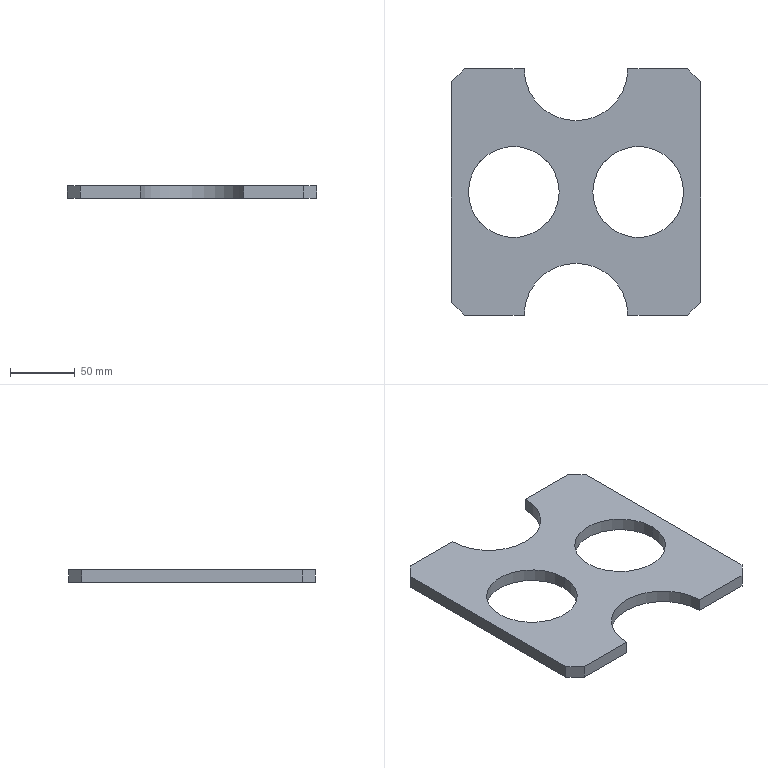Part | SolidWorks | features Extrusion 1 | 1 solid | 18 faces | box 192 x 190 x 10 mm | volume 235565 mm3 | plane 12 | cylinder 6 | commonest cylinder face diameters 70 x4 80 x2
STEP:
#1=CARTESIAN_POINT('',(109.,95.,10.));
#2=VERTEX_POINT('',#1);
#3=CARTESIAN_POINT('',(179.,95.,10.));
#4=VERTEX_POINT('',#3);
#5=CARTESIAN_POINT('',(144.,95.,10.));
#6=DIRECTION('',(0.,0.,1.));
#7=DIRECTION('',(1.,0.,0.));
#8=AXIS2_PLACEMENT_3D('',#5,#6,#7);
#9=CIRCLE('',#8,35.);
#10=EDGE_CURVE('',#2,#4,#9,.T.);
#11=ORIENTED_EDGE('',*,*,#10,.T.);
#12=CARTESIAN_POINT('',(179.,95.,0.));
#13=VERTEX_POINT('',#12);
#14=CARTESIAN_POINT('',(179.,95.,10.));
#15=DIRECTION('',(0.,0.,-1.));
#16=VECTOR('',#15,1000.);
#17=LINE('',#14,#16);
#18=EDGE_CURVE('',#4,#13,#17,.T.);
#19=ORIENTED_EDGE('',*,*,#18,.T.);
#20=CARTESIAN_POINT('',(109.,95.,0.));
#21=VERTEX_POINT('',#20);
#22=CARTESIAN_POINT('',(144.,95.,0.));
#23=DIRECTION('',(0.,0.,1.));
#24=DIRECTION('',(1.,0.,0.));
#25=AXIS2_PLACEMENT_3D('',#22,#23,#24);
#26=CIRCLE('',#25,35.);
#27=EDGE_CURVE('',#21,#13,#26,.T.);
#28=ORIENTED_EDGE('',*,*,#27,.F.);
#29=CARTESIAN_POINT('',(109.,95.,10.));
#30=DIRECTION('',(0.,0.,-1.));
#31=VECTOR('',#30,1000.);
#32=LINE('',#29,#31);
#33=EDGE_CURVE('',#2,#21,#32,.T.);
#34=ORIENTED_EDGE('',*,*,#33,.F.);
#35=EDGE_LOOP('',(#11,#19,#28,#34));
#36=FACE_OUTER_BOUND('',#35,.T.);
#37=CARTESIAN_POINT('',(144.,95.,10.));
#38=DIRECTION('',(0.,0.,-1.));
#39=DIRECTION('',(-1.,0.,0.));
#40=AXIS2_PLACEMENT_3D('',#37,#38,#39);
#41=CYLINDRICAL_SURFACE('',#40,35.);
#42=ADVANCED_FACE('',(#36),#41,.F.);
#43=CARTESIAN_POINT('',(13.,95.,10.));
#44=VERTEX_POINT('',#43);
#45=CARTESIAN_POINT('',(83.,95.,10.));
#46=VERTEX_POINT('',#45);
#47=CARTESIAN_POINT('',(48.,95.,10.));
#48=DIRECTION('',(0.,0.,1.));
#49=DIRECTION('',(1.,0.,0.));
#50=AXIS2_PLACEMENT_3D('',#47,#48,#49);
#51=CIRCLE('',#50,35.);
#52=EDGE_CURVE('',#44,#46,#51,.T.);
#53=ORIENTED_EDGE('',*,*,#52,.T.);
#54=CARTESIAN_POINT('',(83.,95.,0.));
#55=VERTEX_POINT('',#54);
#56=CARTESIAN_POINT('',(83.,95.,10.));
#57=DIRECTION('',(0.,0.,-1.));
#58=VECTOR('',#57,1000.);
#59=LINE('',#56,#58);
#60=EDGE_CURVE('',#46,#55,#59,.T.);
#61=ORIENTED_EDGE('',*,*,#60,.T.);
#62=CARTESIAN_POINT('',(13.,95.,0.));
#63=VERTEX_POINT('',#62);
#64=CARTESIAN_POINT('',(48.,95.,0.));
#65=DIRECTION('',(0.,0.,1.));
#66=DIRECTION('',(1.,0.,0.));
#67=AXIS2_PLACEMENT_3D('',#64,#65,#66);
#68=CIRCLE('',#67,35.);
#69=EDGE_CURVE('',#63,#55,#68,.T.);
#70=ORIENTED_EDGE('',*,*,#69,.F.);
#71=CARTESIAN_POINT('',(13.,95.,10.));
#72=DIRECTION('',(0.,0.,-1.));
#73=VECTOR('',#72,1000.);
#74=LINE('',#71,#73);
#75=EDGE_CURVE('',#44,#63,#74,.T.);
#76=ORIENTED_EDGE('',*,*,#75,.F.);
#77=EDGE_LOOP('',(#53,#61,#70,#76));
#78=FACE_OUTER_BOUND('',#77,.T.);
#79=CARTESIAN_POINT('',(48.,95.,10.));
#80=DIRECTION('',(0.,0.,-1.));
#81=DIRECTION('',(-1.,0.,0.));
#82=AXIS2_PLACEMENT_3D('',#79,#80,#81);
#83=CYLINDRICAL_SURFACE('',#82,35.);
#84=ADVANCED_FACE('',(#78),#83,.F.);
#85=ORIENTED_EDGE('',*,*,#52,.F.);
#86=CARTESIAN_POINT('',(48.,95.,10.));
#87=DIRECTION('',(0.,0.,1.));
#88=DIRECTION('',(1.,0.,0.));
#89=AXIS2_PLACEMENT_3D('',#86,#87,#88);
#90=CIRCLE('',#89,35.);
#91=EDGE_CURVE('',#46,#44,#90,.T.);
#92=ORIENTED_EDGE('',*,*,#91,.F.);
#93=EDGE_LOOP('',(#85,#92));
#94=FACE_BOUND('',#93,.T.);
#95=CARTESIAN_POINT('',(56.,0.,10.));
#96=VERTEX_POINT('',#95);
#97=CARTESIAN_POINT('',(136.,0.,10.));
#98=VERTEX_POINT('',#97);
#99=CARTESIAN_POINT('',(96.,0.,10.));
#100=DIRECTION('',(0.,0.,-1.));
#101=DIRECTION('',(1.,0.,0.));
#102=AXIS2_PLACEMENT_3D('',#99,#100,#101);
#103=CIRCLE('',#102,40.);
#104=EDGE_CURVE('',#96,#98,#103,.T.);
#105=ORIENTED_EDGE('',*,*,#104,.T.);
#106=CARTESIAN_POINT('',(182.,0.,10.));
#107=VERTEX_POINT('',#106);
#108=CARTESIAN_POINT('',(136.,0.,10.));
#109=DIRECTION('',(1.,0.,0.));
#110=VECTOR('',#109,1000.);
#111=LINE('',#108,#110);
#112=EDGE_CURVE('',#98,#107,#111,.T.);
#113=ORIENTED_EDGE('',*,*,#112,.T.);
#114=CARTESIAN_POINT('',(192.,10.,10.));
#115=VERTEX_POINT('',#114);
#116=CARTESIAN_POINT('',(182.,0.,10.));
#117=DIRECTION('',(0.7071,0.7071,0.));
#118=VECTOR('',#117,1000.);
#119=LINE('',#116,#118);
#120=EDGE_CURVE('',#107,#115,#119,.T.);
#121=ORIENTED_EDGE('',*,*,#120,.T.);
#122=CARTESIAN_POINT('',(192.,180.,10.));
#123=VERTEX_POINT('',#122);
#124=CARTESIAN_POINT('',(192.,10.,10.));
#125=DIRECTION('',(0.,1.,0.));
#126=VECTOR('',#125,1000.);
#127=LINE('',#124,#126);
#128=EDGE_CURVE('',#115,#123,#127,.T.);
#129=ORIENTED_EDGE('',*,*,#128,.T.);
#130=CARTESIAN_POINT('',(182.,190.,10.));
#131=VERTEX_POINT('',#130);
#132=CARTESIAN_POINT('',(182.,190.,10.));
#133=DIRECTION('',(-0.7071,0.7071,0.));
#134=VECTOR('',#133,1000.);
#135=LINE('',#132,#134);
#136=EDGE_CURVE('',#123,#131,#135,.T.);
#137=ORIENTED_EDGE('',*,*,#136,.T.);
#138=CARTESIAN_POINT('',(136.,190.,10.));
#139=VERTEX_POINT('',#138);
#140=CARTESIAN_POINT('',(136.,190.,10.));
#141=DIRECTION('',(-1.,0.,0.));
#142=VECTOR('',#141,1000.);
#143=LINE('',#140,#142);
#144=EDGE_CURVE('',#131,#139,#143,.T.);
#145=ORIENTED_EDGE('',*,*,#144,.T.);
#146=CARTESIAN_POINT('',(56.,190.,10.));
#147=VERTEX_POINT('',#146);
#148=CARTESIAN_POINT('',(96.,190.,10.));
#149=DIRECTION('',(0.,0.,-1.));
#150=DIRECTION('',(1.,0.,0.));
#151=AXIS2_PLACEMENT_3D('',#148,#149,#150);
#152=CIRCLE('',#151,40.);
#153=EDGE_CURVE('',#139,#147,#152,.T.);
#154=ORIENTED_EDGE('',*,*,#153,.T.);
#155=CARTESIAN_POINT('',(10.,190.,10.));
#156=VERTEX_POINT('',#155);
#157=CARTESIAN_POINT('',(10.,190.,10.));
#158=DIRECTION('',(-1.,0.,0.));
#159=VECTOR('',#158,1000.);
#160=LINE('',#157,#159);
#161=EDGE_CURVE('',#147,#156,#160,.T.);
#162=ORIENTED_EDGE('',*,*,#161,.T.);
#163=CARTESIAN_POINT('',(0.,180.,10.));
#164=VERTEX_POINT('',#163);
#165=CARTESIAN_POINT('',(0.,180.,10.));
#166=DIRECTION('',(-0.7071,-0.7071,0.));
#167=VECTOR('',#166,1000.);
#168=LINE('',#165,#167);
#169=EDGE_CURVE('',#156,#164,#168,.T.);
#170=ORIENTED_EDGE('',*,*,#169,.T.);
#171=CARTESIAN_POINT('',(0.,10.,10.));
#172=VERTEX_POINT('',#171);
#173=CARTESIAN_POINT('',(0.,10.,10.));
#174=DIRECTION('',(0.,-1.,0.));
#175=VECTOR('',#174,1000.);
#176=LINE('',#173,#175);
#177=EDGE_CURVE('',#164,#172,#176,.T.);
#178=ORIENTED_EDGE('',*,*,#177,.T.);
#179=CARTESIAN_POINT('',(10.,0.,10.));
#180=VERTEX_POINT('',#179);
#181=CARTESIAN_POINT('',(10.,0.,10.));
#182=DIRECTION('',(0.7071,-0.7071,0.));
#183=VECTOR('',#182,1000.);
#184=LINE('',#181,#183);
#185=EDGE_CURVE('',#172,#180,#184,.T.);
#186=ORIENTED_EDGE('',*,*,#185,.T.);
#187=CARTESIAN_POINT('',(10.,0.,10.));
#188=DIRECTION('',(1.,0.,0.));
#189=VECTOR('',#188,1000.);
#190=LINE('',#187,#189);
#191=EDGE_CURVE('',#180,#96,#190,.T.);
#192=ORIENTED_EDGE('',*,*,#191,.T.);
#193=EDGE_LOOP('',(#105,#113,#121,#129,#137,#145,#154,#162,#170,#178,#186,#192));
#194=FACE_OUTER_BOUND('',#193,.T.);
#195=ORIENTED_EDGE('',*,*,#10,.F.);
#196=CARTESIAN_POINT('',(144.,95.,10.));
#197=DIRECTION('',(0.,0.,1.));
#198=DIRECTION('',(1.,0.,0.));
#199=AXIS2_PLACEMENT_3D('',#196,#197,#198);
#200=CIRCLE('',#199,35.);
#201=EDGE_CURVE('',#4,#2,#200,.T.);
#202=ORIENTED_EDGE('',*,*,#201,.F.);
#203=EDGE_LOOP('',(#195,#202));
#204=FACE_BOUND('',#203,.T.);
#205=CARTESIAN_POINT('',(96.,0.,10.));
#206=DIRECTION('',(0.,0.,1.));
#207=DIRECTION('',(1.,0.,0.));
#208=AXIS2_PLACEMENT_3D('',#205,#206,#207);
#209=PLANE('',#208);
#210=ADVANCED_FACE('',(#94,#194,#204),#209,.T.);
#211=ORIENTED_EDGE('',*,*,#69,.T.);
#212=CARTESIAN_POINT('',(48.,95.,0.));
#213=DIRECTION('',(0.,0.,1.));
#214=DIRECTION('',(1.,0.,0.));
#215=AXIS2_PLACEMENT_3D('',#212,#213,#214);
#216=CIRCLE('',#215,35.);
#217=EDGE_CURVE('',#55,#63,#216,.T.);
#218=ORIENTED_EDGE('',*,*,#217,.T.);
#219=EDGE_LOOP('',(#211,#218));
#220=FACE_BOUND('',#219,.T.);
#221=CARTESIAN_POINT('',(56.,0.,0.));
#222=VERTEX_POINT('',#221);
#223=CARTESIAN_POINT('',(136.,0.,0.));
#224=VERTEX_POINT('',#223);
#225=CARTESIAN_POINT('',(96.,0.,0.));
#226=DIRECTION('',(0.,0.,-1.));
#227=DIRECTION('',(1.,0.,0.));
#228=AXIS2_PLACEMENT_3D('',#225,#226,#227);
#229=CIRCLE('',#228,40.);
#230=EDGE_CURVE('',#222,#224,#229,.T.);
#231=ORIENTED_EDGE('',*,*,#230,.F.);
#232=CARTESIAN_POINT('',(10.,0.,0.));
#233=VERTEX_POINT('',#232);
#234=CARTESIAN_POINT('',(10.,0.,0.));
#235=DIRECTION('',(1.,0.,0.));
#236=VECTOR('',#235,1000.);
#237=LINE('',#234,#236);
#238=EDGE_CURVE('',#233,#222,#237,.T.);
#239=ORIENTED_EDGE('',*,*,#238,.F.);
#240=CARTESIAN_POINT('',(0.,10.,0.));
#241=VERTEX_POINT('',#240);
#242=CARTESIAN_POINT('',(10.,0.,0.));
#243=DIRECTION('',(0.7071,-0.7071,0.));
#244=VECTOR('',#243,1000.);
#245=LINE('',#242,#244);
#246=EDGE_CURVE('',#241,#233,#245,.T.);
#247=ORIENTED_EDGE('',*,*,#246,.F.);
#248=CARTESIAN_POINT('',(0.,180.,0.));
#249=VERTEX_POINT('',#248);
#250=CARTESIAN_POINT('',(0.,10.,0.));
#251=DIRECTION('',(0.,-1.,0.));
#252=VECTOR('',#251,1000.);
#253=LINE('',#250,#252);
#254=EDGE_CURVE('',#249,#241,#253,.T.);
#255=ORIENTED_EDGE('',*,*,#254,.F.);
#256=CARTESIAN_POINT('',(10.,190.,0.));
#257=VERTEX_POINT('',#256);
#258=CARTESIAN_POINT('',(0.,180.,0.));
#259=DIRECTION('',(-0.7071,-0.7071,0.));
#260=VECTOR('',#259,1000.);
#261=LINE('',#258,#260);
#262=EDGE_CURVE('',#257,#249,#261,.T.);
#263=ORIENTED_EDGE('',*,*,#262,.F.);
#264=CARTESIAN_POINT('',(56.,190.,0.));
#265=VERTEX_POINT('',#264);
#266=CARTESIAN_POINT('',(10.,190.,0.));
#267=DIRECTION('',(-1.,0.,0.));
#268=VECTOR('',#267,1000.);
#269=LINE('',#266,#268);
#270=EDGE_CURVE('',#265,#257,#269,.T.);
#271=ORIENTED_EDGE('',*,*,#270,.F.);
#272=CARTESIAN_POINT('',(136.,190.,0.));
#273=VERTEX_POINT('',#272);
#274=CARTESIAN_POINT('',(96.,190.,0.));
#275=DIRECTION('',(0.,0.,-1.));
#276=DIRECTION('',(1.,0.,0.));
#277=AXIS2_PLACEMENT_3D('',#274,#275,#276);
#278=CIRCLE('',#277,40.);
#279=EDGE_CURVE('',#273,#265,#278,.T.);
#280=ORIENTED_EDGE('',*,*,#279,.F.);
#281=CARTESIAN_POINT('',(182.,190.,0.));
#282=VERTEX_POINT('',#281);
#283=CARTESIAN_POINT('',(136.,190.,0.));
#284=DIRECTION('',(-1.,0.,0.));
#285=VECTOR('',#284,1000.);
#286=LINE('',#283,#285);
#287=EDGE_CURVE('',#282,#273,#286,.T.);
#288=ORIENTED_EDGE('',*,*,#287,.F.);
#289=CARTESIAN_POINT('',(192.,180.,0.));
#290=VERTEX_POINT('',#289);
#291=CARTESIAN_POINT('',(182.,190.,0.));
#292=DIRECTION('',(-0.7071,0.7071,0.));
#293=VECTOR('',#292,1000.);
#294=LINE('',#291,#293);
#295=EDGE_CURVE('',#290,#282,#294,.T.);
#296=ORIENTED_EDGE('',*,*,#295,.F.);
#297=CARTESIAN_POINT('',(192.,10.,0.));
#298=VERTEX_POINT('',#297);
#299=CARTESIAN_POINT('',(192.,10.,0.));
#300=DIRECTION('',(0.,1.,0.));
#301=VECTOR('',#300,1000.);
#302=LINE('',#299,#301);
#303=EDGE_CURVE('',#298,#290,#302,.T.);
#304=ORIENTED_EDGE('',*,*,#303,.F.);
#305=CARTESIAN_POINT('',(182.,0.,0.));
#306=VERTEX_POINT('',#305);
#307=CARTESIAN_POINT('',(182.,0.,0.));
#308=DIRECTION('',(0.7071,0.7071,0.));
#309=VECTOR('',#308,1000.);
#310=LINE('',#307,#309);
#311=EDGE_CURVE('',#306,#298,#310,.T.);
#312=ORIENTED_EDGE('',*,*,#311,.F.);
#313=CARTESIAN_POINT('',(136.,0.,0.));
#314=DIRECTION('',(1.,0.,0.));
#315=VECTOR('',#314,1000.);
#316=LINE('',#313,#315);
#317=EDGE_CURVE('',#224,#306,#316,.T.);
#318=ORIENTED_EDGE('',*,*,#317,.F.);
#319=EDGE_LOOP('',(#231,#239,#247,#255,#263,#271,#280,#288,#296,#304,#312,#318));
#320=FACE_OUTER_BOUND('',#319,.T.);
#321=ORIENTED_EDGE('',*,*,#27,.T.);
#322=CARTESIAN_POINT('',(144.,95.,0.));
#323=DIRECTION('',(0.,0.,1.));
#324=DIRECTION('',(1.,0.,0.));
#325=AXIS2_PLACEMENT_3D('',#322,#323,#324);
#326=CIRCLE('',#325,35.);
#327=EDGE_CURVE('',#13,#21,#326,.T.);
#328=ORIENTED_EDGE('',*,*,#327,.T.);
#329=EDGE_LOOP('',(#321,#328));
#330=FACE_BOUND('',#329,.T.);
#331=CARTESIAN_POINT('',(96.,0.,0.));
#332=DIRECTION('',(0.,0.,1.));
#333=DIRECTION('',(1.,0.,0.));
#334=AXIS2_PLACEMENT_3D('',#331,#332,#333);
#335=PLANE('',#334);
#336=ADVANCED_FACE('',(#220,#320,#330),#335,.F.);
#337=ORIENTED_EDGE('',*,*,#230,.T.);
#338=CARTESIAN_POINT('',(136.,0.,10.));
#339=DIRECTION('',(0.,0.,-1.));
#340=VECTOR('',#339,1000.);
#341=LINE('',#338,#340);
#342=EDGE_CURVE('',#98,#224,#341,.T.);
#343=ORIENTED_EDGE('',*,*,#342,.F.);
#344=ORIENTED_EDGE('',*,*,#104,.F.);
#345=CARTESIAN_POINT('',(56.,0.,10.));
#346=DIRECTION('',(0.,0.,-1.));
#347=VECTOR('',#346,1000.);
#348=LINE('',#345,#347);
#349=EDGE_CURVE('',#96,#222,#348,.T.);
#350=ORIENTED_EDGE('',*,*,#349,.T.);
#351=EDGE_LOOP('',(#337,#343,#344,#350));
#352=FACE_OUTER_BOUND('',#351,.T.);
#353=CARTESIAN_POINT('',(96.,0.,10.));
#354=DIRECTION('',(0.,0.,-1.));
#355=DIRECTION('',(-1.,0.,0.));
#356=AXIS2_PLACEMENT_3D('',#353,#354,#355);
#357=CYLINDRICAL_SURFACE('',#356,40.);
#358=ADVANCED_FACE('',(#352),#357,.F.);
#359=ORIENTED_EDGE('',*,*,#317,.T.);
#360=CARTESIAN_POINT('',(182.,0.,10.));
#361=DIRECTION('',(0.,0.,-1.));
#362=VECTOR('',#361,1000.);
#363=LINE('',#360,#362);
#364=EDGE_CURVE('',#107,#306,#363,.T.);
#365=ORIENTED_EDGE('',*,*,#364,.F.);
#366=ORIENTED_EDGE('',*,*,#112,.F.);
#367=ORIENTED_EDGE('',*,*,#342,.T.);
#368=EDGE_LOOP('',(#359,#365,#366,#367));
#369=FACE_OUTER_BOUND('',#368,.T.);
#370=CARTESIAN_POINT('',(136.,0.,10.));
#371=DIRECTION('',(0.,1.,0.));
#372=DIRECTION('',(0.,0.,1.));
#373=AXIS2_PLACEMENT_3D('',#370,#371,#372);
#374=PLANE('',#373);
#375=ADVANCED_FACE('',(#369),#374,.F.);
#376=ORIENTED_EDGE('',*,*,#311,.T.);
#377=CARTESIAN_POINT('',(192.,10.,10.));
#378=DIRECTION('',(0.,0.,-1.));
#379=VECTOR('',#378,1000.);
#380=LINE('',#377,#379);
#381=EDGE_CURVE('',#115,#298,#380,.T.);
#382=ORIENTED_EDGE('',*,*,#381,.F.);
#383=ORIENTED_EDGE('',*,*,#120,.F.);
#384=ORIENTED_EDGE('',*,*,#364,.T.);
#385=EDGE_LOOP('',(#376,#382,#383,#384));
#386=FACE_OUTER_BOUND('',#385,.T.);
#387=CARTESIAN_POINT('',(182.,0.,10.));
#388=DIRECTION('',(-0.7071,0.7071,0.));
#389=DIRECTION('',(-0.7071,-0.7071,0.));
#390=AXIS2_PLACEMENT_3D('',#387,#388,#389);
#391=PLANE('',#390);
#392=ADVANCED_FACE('',(#386),#391,.F.);
#393=ORIENTED_EDGE('',*,*,#303,.T.);
#394=CARTESIAN_POINT('',(192.,180.,10.));
#395=DIRECTION('',(0.,0.,-1.));
#396=VECTOR('',#395,1000.);
#397=LINE('',#394,#396);
#398=EDGE_CURVE('',#123,#290,#397,.T.);
#399=ORIENTED_EDGE('',*,*,#398,.F.);
#400=ORIENTED_EDGE('',*,*,#128,.F.);
#401=ORIENTED_EDGE('',*,*,#381,.T.);
#402=EDGE_LOOP('',(#393,#399,#400,#401));
#403=FACE_OUTER_BOUND('',#402,.T.);
#404=CARTESIAN_POINT('',(192.,10.,10.));
#405=DIRECTION('',(-1.,0.,0.));
#406=DIRECTION('',(0.,0.,1.));
#407=AXIS2_PLACEMENT_3D('',#404,#405,#406);
#408=PLANE('',#407);
#409=ADVANCED_FACE('',(#403),#408,.F.);
#410=ORIENTED_EDGE('',*,*,#295,.T.);
#411=CARTESIAN_POINT('',(182.,190.,10.));
#412=DIRECTION('',(0.,0.,-1.));
#413=VECTOR('',#412,1000.);
#414=LINE('',#411,#413);
#415=EDGE_CURVE('',#131,#282,#414,.T.);
#416=ORIENTED_EDGE('',*,*,#415,.F.);
#417=ORIENTED_EDGE('',*,*,#136,.F.);
#418=ORIENTED_EDGE('',*,*,#398,.T.);
#419=EDGE_LOOP('',(#410,#416,#417,#418));
#420=FACE_OUTER_BOUND('',#419,.T.);
#421=CARTESIAN_POINT('',(182.,190.,10.));
#422=DIRECTION('',(-0.7071,-0.7071,0.));
#423=DIRECTION('',(0.7071,-0.7071,0.));
#424=AXIS2_PLACEMENT_3D('',#421,#422,#423);
#425=PLANE('',#424);
#426=ADVANCED_FACE('',(#420),#425,.F.);
#427=ORIENTED_EDGE('',*,*,#287,.T.);
#428=CARTESIAN_POINT('',(136.,190.,10.));
#429=DIRECTION('',(0.,0.,-1.));
#430=VECTOR('',#429,1000.);
#431=LINE('',#428,#430);
#432=EDGE_CURVE('',#139,#273,#431,.T.);
#433=ORIENTED_EDGE('',*,*,#432,.F.);
#434=ORIENTED_EDGE('',*,*,#144,.F.);
#435=ORIENTED_EDGE('',*,*,#415,.T.);
#436=EDGE_LOOP('',(#427,#433,#434,#435));
#437=FACE_OUTER_BOUND('',#436,.T.);
#438=CARTESIAN_POINT('',(136.,190.,10.));
#439=DIRECTION('',(0.,-1.,0.));
#440=DIRECTION('',(0.,0.,-1.));
#441=AXIS2_PLACEMENT_3D('',#438,#439,#440);
#442=PLANE('',#441);
#443=ADVANCED_FACE('',(#437),#442,.F.);
#444=ORIENTED_EDGE('',*,*,#279,.T.);
#445=CARTESIAN_POINT('',(56.,190.,10.));
#446=DIRECTION('',(0.,0.,-1.));
#447=VECTOR('',#446,1000.);
#448=LINE('',#445,#447);
#449=EDGE_CURVE('',#147,#265,#448,.T.);
#450=ORIENTED_EDGE('',*,*,#449,.F.);
#451=ORIENTED_EDGE('',*,*,#153,.F.);
#452=ORIENTED_EDGE('',*,*,#432,.T.);
#453=EDGE_LOOP('',(#444,#450,#451,#452));
#454=FACE_OUTER_BOUND('',#453,.T.);
#455=CARTESIAN_POINT('',(96.,190.,10.));
#456=DIRECTION('',(0.,0.,-1.));
#457=DIRECTION('',(-1.,0.,0.));
#458=AXIS2_PLACEMENT_3D('',#455,#456,#457);
#459=CYLINDRICAL_SURFACE('',#458,40.);
#460=ADVANCED_FACE('',(#454),#459,.F.);
#461=ORIENTED_EDGE('',*,*,#270,.T.);
#462=CARTESIAN_POINT('',(10.,190.,10.));
#463=DIRECTION('',(0.,0.,-1.));
#464=VECTOR('',#463,1000.);
#465=LINE('',#462,#464);
#466=EDGE_CURVE('',#156,#257,#465,.T.);
#467=ORIENTED_EDGE('',*,*,#466,.F.);
#468=ORIENTED_EDGE('',*,*,#161,.F.);
#469=ORIENTED_EDGE('',*,*,#449,.T.);
#470=EDGE_LOOP('',(#461,#467,#468,#469));
#471=FACE_OUTER_BOUND('',#470,.T.);
#472=CARTESIAN_POINT('',(10.,190.,10.));
#473=DIRECTION('',(0.,-1.,0.));
#474=DIRECTION('',(0.,0.,-1.));
#475=AXIS2_PLACEMENT_3D('',#472,#473,#474);
#476=PLANE('',#475);
#477=ADVANCED_FACE('',(#471),#476,.F.);
#478=ORIENTED_EDGE('',*,*,#262,.T.);
#479=CARTESIAN_POINT('',(0.,180.,10.));
#480=DIRECTION('',(0.,0.,-1.));
#481=VECTOR('',#480,1000.);
#482=LINE('',#479,#481);
#483=EDGE_CURVE('',#164,#249,#482,.T.);
#484=ORIENTED_EDGE('',*,*,#483,.F.);
#485=ORIENTED_EDGE('',*,*,#169,.F.);
#486=ORIENTED_EDGE('',*,*,#466,.T.);
#487=EDGE_LOOP('',(#478,#484,#485,#486));
#488=FACE_OUTER_BOUND('',#487,.T.);
#489=CARTESIAN_POINT('',(0.,180.,10.));
#490=DIRECTION('',(0.7071,-0.7071,0.));
#491=DIRECTION('',(0.7071,0.7071,0.));
#492=AXIS2_PLACEMENT_3D('',#489,#490,#491);
#493=PLANE('',#492);
#494=ADVANCED_FACE('',(#488),#493,.F.);
#495=ORIENTED_EDGE('',*,*,#254,.T.);
#496=CARTESIAN_POINT('',(0.,10.,10.));
#497=DIRECTION('',(0.,0.,-1.));
#498=VECTOR('',#497,1000.);
#499=LINE('',#496,#498);
#500=EDGE_CURVE('',#172,#241,#499,.T.);
#501=ORIENTED_EDGE('',*,*,#500,.F.);
#502=ORIENTED_EDGE('',*,*,#177,.F.);
#503=ORIENTED_EDGE('',*,*,#483,.T.);
#504=EDGE_LOOP('',(#495,#501,#502,#503));
#505=FACE_OUTER_BOUND('',#504,.T.);
#506=CARTESIAN_POINT('',(0.,10.,10.));
#507=DIRECTION('',(1.,0.,0.));
#508=DIRECTION('',(0.,0.,-1.));
#509=AXIS2_PLACEMENT_3D('',#506,#507,#508);
#510=PLANE('',#509);
#511=ADVANCED_FACE('',(#505),#510,.F.);
#512=ORIENTED_EDGE('',*,*,#246,.T.);
#513=CARTESIAN_POINT('',(10.,0.,10.));
#514=DIRECTION('',(0.,0.,-1.));
#515=VECTOR('',#514,1000.);
#516=LINE('',#513,#515);
#517=EDGE_CURVE('',#180,#233,#516,.T.);
#518=ORIENTED_EDGE('',*,*,#517,.F.);
#519=ORIENTED_EDGE('',*,*,#185,.F.);
#520=ORIENTED_EDGE('',*,*,#500,.T.);
#521=EDGE_LOOP('',(#512,#518,#519,#520));
#522=FACE_OUTER_BOUND('',#521,.T.);
#523=CARTESIAN_POINT('',(10.,0.,10.));
#524=DIRECTION('',(0.7071,0.7071,0.));
#525=DIRECTION('',(-0.7071,0.7071,0.));
#526=AXIS2_PLACEMENT_3D('',#523,#524,#525);
#527=PLANE('',#526);
#528=ADVANCED_FACE('',(#522),#527,.F.);
#529=ORIENTED_EDGE('',*,*,#238,.T.);
#530=ORIENTED_EDGE('',*,*,#349,.F.);
#531=ORIENTED_EDGE('',*,*,#191,.F.);
#532=ORIENTED_EDGE('',*,*,#517,.T.);
#533=EDGE_LOOP('',(#529,#530,#531,#532));
#534=FACE_OUTER_BOUND('',#533,.T.);
#535=CARTESIAN_POINT('',(10.,0.,10.));
#536=DIRECTION('',(0.,1.,0.));
#537=DIRECTION('',(0.,0.,1.));
#538=AXIS2_PLACEMENT_3D('',#535,#536,#537);
#539=PLANE('',#538);
#540=ADVANCED_FACE('',(#534),#539,.F.);
#541=ORIENTED_EDGE('',*,*,#60,.F.);
#542=ORIENTED_EDGE('',*,*,#91,.T.);
#543=ORIENTED_EDGE('',*,*,#75,.T.);
#544=ORIENTED_EDGE('',*,*,#217,.F.);
#545=EDGE_LOOP('',(#541,#542,#543,#544));
#546=FACE_OUTER_BOUND('',#545,.T.);
#547=CARTESIAN_POINT('',(48.,95.,10.));
#548=DIRECTION('',(0.,0.,-1.));
#549=DIRECTION('',(-1.,0.,0.));
#550=AXIS2_PLACEMENT_3D('',#547,#548,#549);
#551=CYLINDRICAL_SURFACE('',#550,35.);
#552=ADVANCED_FACE('',(#546),#551,.F.);
#553=ORIENTED_EDGE('',*,*,#18,.F.);
#554=ORIENTED_EDGE('',*,*,#201,.T.);
#555=ORIENTED_EDGE('',*,*,#33,.T.);
#556=ORIENTED_EDGE('',*,*,#327,.F.);
#557=EDGE_LOOP('',(#553,#554,#555,#556));
#558=FACE_OUTER_BOUND('',#557,.T.);
#559=CARTESIAN_POINT('',(144.,95.,10.));
#560=DIRECTION('',(0.,0.,-1.));
#561=DIRECTION('',(-1.,0.,0.));
#562=AXIS2_PLACEMENT_3D('',#559,#560,#561);
#563=CYLINDRICAL_SURFACE('',#562,35.);
#564=ADVANCED_FACE('',(#558),#563,.F.);
#565=CLOSED_SHELL('',(#42,#84,#210,#336,#358,#375,#392,#409,#426,#443,#460,#477,#494,#511,#528,#540,#552,#564));
#566=MANIFOLD_SOLID_BREP('',#565);
#567=CARTESIAN_POINT('',(0.,0.,0.));
#568=DIRECTION('',(0.,0.,1.));
#569=DIRECTION('',(1.,0.,0.));
#570=AXIS2_PLACEMENT_3D('',#567,#568,#569);
#571=(LENGTH_UNIT()NAMED_UNIT(*)SI_UNIT(.MILLI.,.METRE.));
#572=UNCERTAINTY_MEASURE_WITH_UNIT(LENGTH_MEASURE(0.00001),#571,'','');
#573=(NAMED_UNIT(*)PLANE_ANGLE_UNIT()SI_UNIT($,.RADIAN.));
#574=(NAMED_UNIT(*)SI_UNIT($,.STERADIAN.)SOLID_ANGLE_UNIT());
#575=(GEOMETRIC_REPRESENTATION_CONTEXT(3)GLOBAL_UNCERTAINTY_ASSIGNED_CONTEXT((#572))GLOBAL_UNIT_ASSIGNED_CONTEXT((#571,#573,#574))REPRESENTATION_CONTEXT('',''));
#576=ADVANCED_BREP_SHAPE_REPRESENTATION('',(#566,#570),#575);